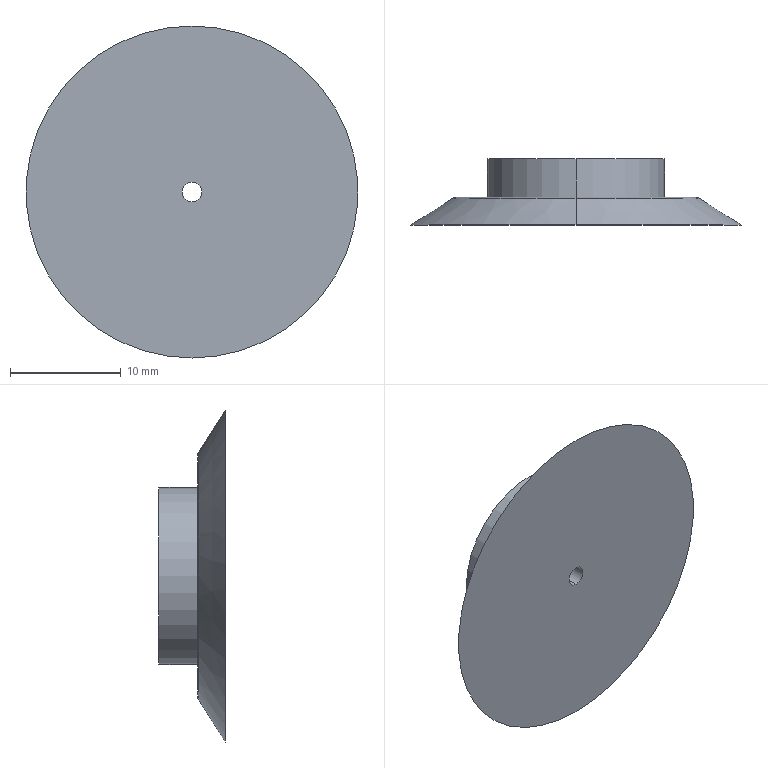Part | SolidWorks | features HoleWzd 1, Revolution 1 | 1 solid | 11 faces | box 30 x 6 x 30 mm | volume 2026 mm3 | cylinder 4 | plane 3 | cone 2 | torus 2 | commonest cylinder face diameters 1.8 x2 16 x2
STEP:
#1=CARTESIAN_POINT('',(0.,-9.454,0.9));
#2=VERTEX_POINT('',#1);
#3=CARTESIAN_POINT('',(0.,-9.454,-0.9));
#4=VERTEX_POINT('',#3);
#5=CARTESIAN_POINT('',(0.,-9.454,0.));
#6=DIRECTION('',(0.,-1.,0.));
#7=DIRECTION('',(0.,0.,-1.));
#8=AXIS2_PLACEMENT_3D('',#5,#6,#7);
#9=CIRCLE('',#8,0.9);
#10=EDGE_CURVE('',#2,#4,#9,.T.);
#11=ORIENTED_EDGE('',*,*,#10,.F.);
#12=CARTESIAN_POINT('',(0.,-15.454,0.9));
#13=VERTEX_POINT('',#12);
#14=CARTESIAN_POINT('',(0.,-15.454,0.9));
#15=DIRECTION('',(0.,-1.,0.));
#16=VECTOR('',#15,1000.);
#17=LINE('',#14,#16);
#18=EDGE_CURVE('',#2,#13,#17,.T.);
#19=ORIENTED_EDGE('',*,*,#18,.T.);
#20=CARTESIAN_POINT('',(0.,-15.454,-0.9));
#21=VERTEX_POINT('',#20);
#22=CARTESIAN_POINT('',(0.,-15.454,0.));
#23=DIRECTION('',(0.,-1.,0.));
#24=DIRECTION('',(0.,0.,-1.));
#25=AXIS2_PLACEMENT_3D('',#22,#23,#24);
#26=CIRCLE('',#25,0.9);
#27=EDGE_CURVE('',#13,#21,#26,.T.);
#28=ORIENTED_EDGE('',*,*,#27,.T.);
#29=CARTESIAN_POINT('',(0.,-15.454,-0.9));
#30=DIRECTION('',(0.,-1.,0.));
#31=VECTOR('',#30,1000.);
#32=LINE('',#29,#31);
#33=EDGE_CURVE('',#4,#21,#32,.T.);
#34=ORIENTED_EDGE('',*,*,#33,.F.);
#35=EDGE_LOOP('',(#11,#19,#28,#34));
#36=FACE_OUTER_BOUND('',#35,.T.);
#37=CARTESIAN_POINT('',(0.,-15.454,0.));
#38=DIRECTION('',(0.,-1.,0.));
#39=DIRECTION('',(0.,0.,-1.));
#40=AXIS2_PLACEMENT_3D('',#37,#38,#39);
#41=CYLINDRICAL_SURFACE('',#40,0.9);
#42=ADVANCED_FACE('',(#36),#41,.F.);
#43=CARTESIAN_POINT('',(0.,-13.03,11.122));
#44=VERTEX_POINT('',#43);
#45=CARTESIAN_POINT('',(0.,-13.03,-11.122));
#46=VERTEX_POINT('',#45);
#47=CARTESIAN_POINT('',(0.,-13.03,0.));
#48=DIRECTION('',(0.,1.,0.));
#49=DIRECTION('',(0.,0.,1.));
#50=AXIS2_PLACEMENT_3D('',#47,#48,#49);
#51=CIRCLE('',#50,11.122);
#52=EDGE_CURVE('',#44,#46,#51,.T.);
#53=ORIENTED_EDGE('',*,*,#52,.F.);
#54=CARTESIAN_POINT('',(0.,-15.454,15.));
#55=VERTEX_POINT('',#54);
#56=CARTESIAN_POINT('',(0.,-13.03,11.122));
#57=DIRECTION('',(0.,-0.53,0.848));
#58=VECTOR('',#57,1000.);
#59=LINE('',#56,#58);
#60=EDGE_CURVE('',#44,#55,#59,.T.);
#61=ORIENTED_EDGE('',*,*,#60,.T.);
#62=CARTESIAN_POINT('',(0.,-15.454,-15.));
#63=VERTEX_POINT('',#62);
#64=CARTESIAN_POINT('',(0.,-15.454,0.));
#65=DIRECTION('',(0.,1.,0.));
#66=DIRECTION('',(0.,0.,1.));
#67=AXIS2_PLACEMENT_3D('',#64,#65,#66);
#68=CIRCLE('',#67,15.);
#69=EDGE_CURVE('',#55,#63,#68,.T.);
#70=ORIENTED_EDGE('',*,*,#69,.T.);
#71=CARTESIAN_POINT('',(0.,-13.03,-11.122));
#72=DIRECTION('',(0.,-0.53,-0.848));
#73=VECTOR('',#72,1000.);
#74=LINE('',#71,#73);
#75=EDGE_CURVE('',#46,#63,#74,.T.);
#76=ORIENTED_EDGE('',*,*,#75,.F.);
#77=EDGE_LOOP('',(#53,#61,#70,#76));
#78=FACE_OUTER_BOUND('',#77,.T.);
#79=CARTESIAN_POINT('',(0.,-13.03,0.));
#80=DIRECTION('',(0.,-1.,0.));
#81=DIRECTION('',(0.,0.,-1.));
#82=AXIS2_PLACEMENT_3D('',#79,#80,#81);
#83=CONICAL_SURFACE('',#82,11.122,1.012);
#84=ADVANCED_FACE('',(#78),#83,.T.);
#85=ORIENTED_EDGE('',*,*,#52,.T.);
#86=CARTESIAN_POINT('',(0.,-12.954,-10.857));
#87=VERTEX_POINT('',#86);
#88=CARTESIAN_POINT('',(0.,-13.454,-10.857));
#89=DIRECTION('',(1.,0.,0.));
#90=DIRECTION('',(0.,0.,-1.));
#91=AXIS2_PLACEMENT_3D('',#88,#89,#90);
#92=CIRCLE('',#91,0.5);
#93=EDGE_CURVE('',#46,#87,#92,.T.);
#94=ORIENTED_EDGE('',*,*,#93,.T.);
#95=CARTESIAN_POINT('',(0.,-12.954,10.857));
#96=VERTEX_POINT('',#95);
#97=CARTESIAN_POINT('',(0.,-12.954,0.));
#98=DIRECTION('',(0.,1.,0.));
#99=DIRECTION('',(0.,0.,1.));
#100=AXIS2_PLACEMENT_3D('',#97,#98,#99);
#101=CIRCLE('',#100,10.857);
#102=EDGE_CURVE('',#96,#87,#101,.T.);
#103=ORIENTED_EDGE('',*,*,#102,.F.);
#104=CARTESIAN_POINT('',(0.,-13.454,10.857));
#105=DIRECTION('',(-1.,0.,0.));
#106=DIRECTION('',(0.,0.,1.));
#107=AXIS2_PLACEMENT_3D('',#104,#105,#106);
#108=CIRCLE('',#107,0.5);
#109=EDGE_CURVE('',#44,#96,#108,.T.);
#110=ORIENTED_EDGE('',*,*,#109,.F.);
#111=EDGE_LOOP('',(#85,#94,#103,#110));
#112=FACE_OUTER_BOUND('',#111,.T.);
#113=CARTESIAN_POINT('',(0.,-13.454,0.));
#114=DIRECTION('',(0.,1.,0.));
#115=DIRECTION('',(0.,0.,1.));
#116=AXIS2_PLACEMENT_3D('',#113,#114,#115);
#117=TOROIDAL_SURFACE('',#116,10.857,0.5);
#118=ADVANCED_FACE('',(#112),#117,.T.);
#119=CARTESIAN_POINT('',(0.,-12.954,8.));
#120=VERTEX_POINT('',#119);
#121=CARTESIAN_POINT('',(0.,-12.954,-8.));
#122=VERTEX_POINT('',#121);
#123=CARTESIAN_POINT('',(0.,-12.954,0.));
#124=DIRECTION('',(0.,1.,0.));
#125=DIRECTION('',(0.,0.,1.));
#126=AXIS2_PLACEMENT_3D('',#123,#124,#125);
#127=CIRCLE('',#126,8.);
#128=EDGE_CURVE('',#120,#122,#127,.T.);
#129=ORIENTED_EDGE('',*,*,#128,.T.);
#130=CARTESIAN_POINT('',(0.,-9.454,-8.));
#131=VERTEX_POINT('',#130);
#132=CARTESIAN_POINT('',(0.,20.859,-8.));
#133=DIRECTION('',(0.,1.,0.));
#134=VECTOR('',#133,1000.);
#135=LINE('',#132,#134);
#136=EDGE_CURVE('',#122,#131,#135,.T.);
#137=ORIENTED_EDGE('',*,*,#136,.T.);
#138=CARTESIAN_POINT('',(0.,-9.454,8.));
#139=VERTEX_POINT('',#138);
#140=CARTESIAN_POINT('',(0.,-9.454,0.));
#141=DIRECTION('',(0.,1.,0.));
#142=DIRECTION('',(0.,0.,1.));
#143=AXIS2_PLACEMENT_3D('',#140,#141,#142);
#144=CIRCLE('',#143,8.);
#145=EDGE_CURVE('',#139,#131,#144,.T.);
#146=ORIENTED_EDGE('',*,*,#145,.F.);
#147=CARTESIAN_POINT('',(0.,20.859,8.));
#148=DIRECTION('',(0.,1.,0.));
#149=VECTOR('',#148,1000.);
#150=LINE('',#147,#149);
#151=EDGE_CURVE('',#120,#139,#150,.T.);
#152=ORIENTED_EDGE('',*,*,#151,.F.);
#153=EDGE_LOOP('',(#129,#137,#146,#152));
#154=FACE_OUTER_BOUND('',#153,.T.);
#155=CARTESIAN_POINT('',(0.,20.859,0.));
#156=DIRECTION('',(0.,1.,0.));
#157=DIRECTION('',(0.,0.,1.));
#158=AXIS2_PLACEMENT_3D('',#155,#156,#157);
#159=CYLINDRICAL_SURFACE('',#158,8.);
#160=ADVANCED_FACE('',(#154),#159,.T.);
#161=CARTESIAN_POINT('',(0.,-9.454,0.));
#162=DIRECTION('',(0.,-1.,0.));
#163=DIRECTION('',(0.,0.,-1.));
#164=AXIS2_PLACEMENT_3D('',#161,#162,#163);
#165=CIRCLE('',#164,0.9);
#166=EDGE_CURVE('',#4,#2,#165,.T.);
#167=ORIENTED_EDGE('',*,*,#166,.T.);
#168=ORIENTED_EDGE('',*,*,#10,.T.);
#169=EDGE_LOOP('',(#167,#168));
#170=FACE_BOUND('',#169,.T.);
#171=ORIENTED_EDGE('',*,*,#145,.T.);
#172=CARTESIAN_POINT('',(0.,-9.454,0.));
#173=DIRECTION('',(0.,1.,0.));
#174=DIRECTION('',(0.,0.,1.));
#175=AXIS2_PLACEMENT_3D('',#172,#173,#174);
#176=CIRCLE('',#175,8.);
#177=EDGE_CURVE('',#131,#139,#176,.T.);
#178=ORIENTED_EDGE('',*,*,#177,.T.);
#179=EDGE_LOOP('',(#171,#178));
#180=FACE_OUTER_BOUND('',#179,.T.);
#181=CARTESIAN_POINT('',(-8.,-9.454,0.));
#182=DIRECTION('',(0.,1.,0.));
#183=DIRECTION('',(0.,0.,1.));
#184=AXIS2_PLACEMENT_3D('',#181,#182,#183);
#185=PLANE('',#184);
#186=ADVANCED_FACE('',(#170,#180),#185,.T.);
#187=ORIENTED_EDGE('',*,*,#136,.F.);
#188=CARTESIAN_POINT('',(0.,-12.954,0.));
#189=DIRECTION('',(0.,1.,0.));
#190=DIRECTION('',(0.,0.,1.));
#191=AXIS2_PLACEMENT_3D('',#188,#189,#190);
#192=CIRCLE('',#191,8.);
#193=EDGE_CURVE('',#122,#120,#192,.T.);
#194=ORIENTED_EDGE('',*,*,#193,.T.);
#195=ORIENTED_EDGE('',*,*,#151,.T.);
#196=ORIENTED_EDGE('',*,*,#177,.F.);
#197=EDGE_LOOP('',(#187,#194,#195,#196));
#198=FACE_OUTER_BOUND('',#197,.T.);
#199=CARTESIAN_POINT('',(0.,20.859,0.));
#200=DIRECTION('',(0.,1.,0.));
#201=DIRECTION('',(0.,0.,1.));
#202=AXIS2_PLACEMENT_3D('',#199,#200,#201);
#203=CYLINDRICAL_SURFACE('',#202,8.);
#204=ADVANCED_FACE('',(#198),#203,.T.);
#205=ORIENTED_EDGE('',*,*,#102,.T.);
#206=CARTESIAN_POINT('',(0.,-12.954,0.));
#207=DIRECTION('',(0.,1.,0.));
#208=DIRECTION('',(0.,0.,1.));
#209=AXIS2_PLACEMENT_3D('',#206,#207,#208);
#210=CIRCLE('',#209,10.857);
#211=EDGE_CURVE('',#87,#96,#210,.T.);
#212=ORIENTED_EDGE('',*,*,#211,.T.);
#213=EDGE_LOOP('',(#205,#212));
#214=FACE_OUTER_BOUND('',#213,.T.);
#215=ORIENTED_EDGE('',*,*,#128,.F.);
#216=ORIENTED_EDGE('',*,*,#193,.F.);
#217=EDGE_LOOP('',(#215,#216));
#218=FACE_BOUND('',#217,.T.);
#219=CARTESIAN_POINT('',(-10.857,-12.954,0.));
#220=DIRECTION('',(0.,1.,0.));
#221=DIRECTION('',(0.,0.,1.));
#222=AXIS2_PLACEMENT_3D('',#219,#220,#221);
#223=PLANE('',#222);
#224=ADVANCED_FACE('',(#214,#218),#223,.T.);
#225=ORIENTED_EDGE('',*,*,#93,.F.);
#226=CARTESIAN_POINT('',(0.,-13.03,0.));
#227=DIRECTION('',(0.,1.,0.));
#228=DIRECTION('',(0.,0.,1.));
#229=AXIS2_PLACEMENT_3D('',#226,#227,#228);
#230=CIRCLE('',#229,11.122);
#231=EDGE_CURVE('',#46,#44,#230,.T.);
#232=ORIENTED_EDGE('',*,*,#231,.T.);
#233=ORIENTED_EDGE('',*,*,#109,.T.);
#234=ORIENTED_EDGE('',*,*,#211,.F.);
#235=EDGE_LOOP('',(#225,#232,#233,#234));
#236=FACE_OUTER_BOUND('',#235,.T.);
#237=CARTESIAN_POINT('',(0.,-13.454,0.));
#238=DIRECTION('',(0.,1.,0.));
#239=DIRECTION('',(0.,0.,1.));
#240=AXIS2_PLACEMENT_3D('',#237,#238,#239);
#241=TOROIDAL_SURFACE('',#240,10.857,0.5);
#242=ADVANCED_FACE('',(#236),#241,.T.);
#243=ORIENTED_EDGE('',*,*,#60,.F.);
#244=ORIENTED_EDGE('',*,*,#231,.F.);
#245=ORIENTED_EDGE('',*,*,#75,.T.);
#246=CARTESIAN_POINT('',(0.,-15.454,0.));
#247=DIRECTION('',(0.,1.,0.));
#248=DIRECTION('',(0.,0.,1.));
#249=AXIS2_PLACEMENT_3D('',#246,#247,#248);
#250=CIRCLE('',#249,15.);
#251=EDGE_CURVE('',#63,#55,#250,.T.);
#252=ORIENTED_EDGE('',*,*,#251,.T.);
#253=EDGE_LOOP('',(#243,#244,#245,#252));
#254=FACE_OUTER_BOUND('',#253,.T.);
#255=CARTESIAN_POINT('',(0.,-13.03,0.));
#256=DIRECTION('',(0.,-1.,0.));
#257=DIRECTION('',(0.,0.,-1.));
#258=AXIS2_PLACEMENT_3D('',#255,#256,#257);
#259=CONICAL_SURFACE('',#258,11.122,1.012);
#260=ADVANCED_FACE('',(#254),#259,.T.);
#261=CARTESIAN_POINT('',(0.,-15.454,0.));
#262=DIRECTION('',(0.,-1.,0.));
#263=DIRECTION('',(0.,0.,-1.));
#264=AXIS2_PLACEMENT_3D('',#261,#262,#263);
#265=CIRCLE('',#264,0.9);
#266=EDGE_CURVE('',#21,#13,#265,.T.);
#267=ORIENTED_EDGE('',*,*,#266,.F.);
#268=ORIENTED_EDGE('',*,*,#27,.F.);
#269=EDGE_LOOP('',(#267,#268));
#270=FACE_BOUND('',#269,.T.);
#271=ORIENTED_EDGE('',*,*,#251,.F.);
#272=ORIENTED_EDGE('',*,*,#69,.F.);
#273=EDGE_LOOP('',(#271,#272));
#274=FACE_OUTER_BOUND('',#273,.T.);
#275=CARTESIAN_POINT('',(0.,-15.454,0.));
#276=DIRECTION('',(0.,-1.,0.));
#277=DIRECTION('',(0.,0.,-1.));
#278=AXIS2_PLACEMENT_3D('',#275,#276,#277);
#279=PLANE('',#278);
#280=ADVANCED_FACE('',(#270,#274),#279,.T.);
#281=ORIENTED_EDGE('',*,*,#18,.F.);
#282=ORIENTED_EDGE('',*,*,#166,.F.);
#283=ORIENTED_EDGE('',*,*,#33,.T.);
#284=ORIENTED_EDGE('',*,*,#266,.T.);
#285=EDGE_LOOP('',(#281,#282,#283,#284));
#286=FACE_OUTER_BOUND('',#285,.T.);
#287=CARTESIAN_POINT('',(0.,-15.454,0.));
#288=DIRECTION('',(0.,-1.,0.));
#289=DIRECTION('',(0.,0.,-1.));
#290=AXIS2_PLACEMENT_3D('',#287,#288,#289);
#291=CYLINDRICAL_SURFACE('',#290,0.9);
#292=ADVANCED_FACE('',(#286),#291,.F.);
#293=CLOSED_SHELL('',(#42,#84,#118,#160,#186,#204,#224,#242,#260,#280,#292));
#294=MANIFOLD_SOLID_BREP('',#293);
#295=CARTESIAN_POINT('',(0.,0.,0.));
#296=DIRECTION('',(0.,0.,1.));
#297=DIRECTION('',(1.,0.,0.));
#298=AXIS2_PLACEMENT_3D('',#295,#296,#297);
#299=(LENGTH_UNIT()NAMED_UNIT(*)SI_UNIT(.MILLI.,.METRE.));
#300=UNCERTAINTY_MEASURE_WITH_UNIT(LENGTH_MEASURE(0.00001),#299,'','');
#301=(NAMED_UNIT(*)PLANE_ANGLE_UNIT()SI_UNIT($,.RADIAN.));
#302=(NAMED_UNIT(*)SI_UNIT($,.STERADIAN.)SOLID_ANGLE_UNIT());
#303=(GEOMETRIC_REPRESENTATION_CONTEXT(3)GLOBAL_UNCERTAINTY_ASSIGNED_CONTEXT((#300))GLOBAL_UNIT_ASSIGNED_CONTEXT((#299,#301,#302))REPRESENTATION_CONTEXT('',''));
#304=ADVANCED_BREP_SHAPE_REPRESENTATION('',(#294,#298),#303);